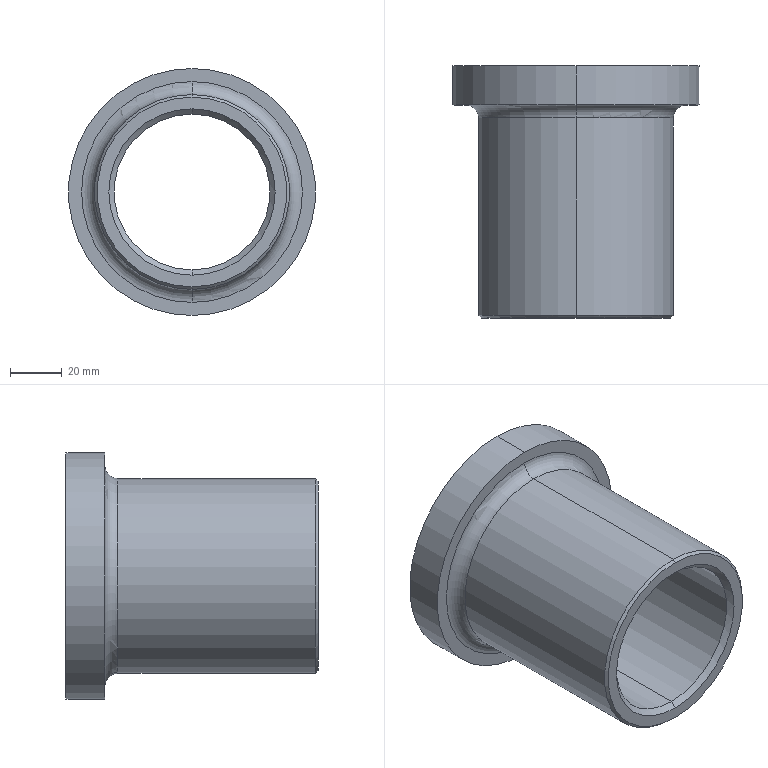Part | SolidWorks | features Chamfer 3, Extrusion 1, Fillet 1, ICE 1 | 1 solid | 17 faces | box 95 x 97 x 95 mm | volume 192640 mm3 | cone 6 | cylinder 6 | plane 3 | torus 2 | commonest cylinder face diameters 60 x2 75 x2 95 x2
STEP:
#1=CARTESIAN_POINT('',(0.,-82.,-36.5));
#2=VERTEX_POINT('',#1);
#3=CARTESIAN_POINT('',(0.,-82.,36.5));
#4=VERTEX_POINT('',#3);
#5=CARTESIAN_POINT('',(0.,-82.,0.));
#6=DIRECTION('',(0.,-1.,0.));
#7=DIRECTION('',(0.,0.,-1.));
#8=AXIS2_PLACEMENT_3D('',#5,#6,#7);
#9=CIRCLE('',#8,36.5);
#10=EDGE_CURVE('',#2,#4,#9,.T.);
#11=ORIENTED_EDGE('',*,*,#10,.F.);
#12=CARTESIAN_POINT('',(0.,-81.,-37.5));
#13=VERTEX_POINT('',#12);
#14=CARTESIAN_POINT('',(0.,-82.,-36.5));
#15=DIRECTION('',(0.,0.7071,-0.7071));
#16=VECTOR('',#15,1000.);
#17=LINE('',#14,#16);
#18=EDGE_CURVE('',#2,#13,#17,.T.);
#19=ORIENTED_EDGE('',*,*,#18,.T.);
#20=CARTESIAN_POINT('',(0.,-81.,37.5));
#21=VERTEX_POINT('',#20);
#22=CARTESIAN_POINT('',(0.,-81.,0.));
#23=DIRECTION('',(0.,1.,0.));
#24=DIRECTION('',(0.,0.,-1.));
#25=AXIS2_PLACEMENT_3D('',#22,#23,#24);
#26=CIRCLE('',#25,37.5);
#27=EDGE_CURVE('',#21,#13,#26,.T.);
#28=ORIENTED_EDGE('',*,*,#27,.F.);
#29=CARTESIAN_POINT('',(0.,-82.,36.5));
#30=DIRECTION('',(0.,0.7071,0.7071));
#31=VECTOR('',#30,1000.);
#32=LINE('',#29,#31);
#33=EDGE_CURVE('',#4,#21,#32,.T.);
#34=ORIENTED_EDGE('',*,*,#33,.F.);
#35=EDGE_LOOP('',(#11,#19,#28,#34));
#36=FACE_OUTER_BOUND('',#35,.T.);
#37=CARTESIAN_POINT('',(0.,-82.,0.));
#38=DIRECTION('',(0.,1.,0.));
#39=DIRECTION('',(0.,0.,1.));
#40=AXIS2_PLACEMENT_3D('',#37,#38,#39);
#41=CONICAL_SURFACE('',#40,36.5,0.7854);
#42=ADVANCED_FACE('',(#36),#41,.T.);
#43=CARTESIAN_POINT('',(0.,10.,-30.));
#44=VERTEX_POINT('',#43);
#45=CARTESIAN_POINT('',(0.,10.,30.));
#46=VERTEX_POINT('',#45);
#47=CARTESIAN_POINT('',(0.,10.,0.));
#48=DIRECTION('',(0.,1.,0.));
#49=DIRECTION('',(0.,0.,1.));
#50=AXIS2_PLACEMENT_3D('',#47,#48,#49);
#51=CIRCLE('',#50,30.);
#52=EDGE_CURVE('',#44,#46,#51,.T.);
#53=ORIENTED_EDGE('',*,*,#52,.F.);
#54=CARTESIAN_POINT('',(0.,15.,-35.));
#55=VERTEX_POINT('',#54);
#56=CARTESIAN_POINT('',(0.,10.,-30.));
#57=DIRECTION('',(0.,0.7071,-0.7071));
#58=VECTOR('',#57,1000.);
#59=LINE('',#56,#58);
#60=EDGE_CURVE('',#44,#55,#59,.T.);
#61=ORIENTED_EDGE('',*,*,#60,.T.);
#62=CARTESIAN_POINT('',(0.,15.,35.));
#63=VERTEX_POINT('',#62);
#64=CARTESIAN_POINT('',(0.,15.,0.));
#65=DIRECTION('',(0.,-1.,0.));
#66=DIRECTION('',(0.,0.,1.));
#67=AXIS2_PLACEMENT_3D('',#64,#65,#66);
#68=CIRCLE('',#67,35.);
#69=EDGE_CURVE('',#63,#55,#68,.T.);
#70=ORIENTED_EDGE('',*,*,#69,.F.);
#71=CARTESIAN_POINT('',(0.,10.,30.));
#72=DIRECTION('',(0.,0.7071,0.7071));
#73=VECTOR('',#72,1000.);
#74=LINE('',#71,#73);
#75=EDGE_CURVE('',#46,#63,#74,.T.);
#76=ORIENTED_EDGE('',*,*,#75,.F.);
#77=EDGE_LOOP('',(#53,#61,#70,#76));
#78=FACE_OUTER_BOUND('',#77,.T.);
#79=CARTESIAN_POINT('',(0.,10.,0.));
#80=DIRECTION('',(0.,1.,0.));
#81=DIRECTION('',(0.,0.,1.));
#82=AXIS2_PLACEMENT_3D('',#79,#80,#81);
#83=CONICAL_SURFACE('',#82,30.,0.7854);
#84=ADVANCED_FACE('',(#78),#83,.F.);
#85=CARTESIAN_POINT('',(0.,-80.,30.));
#86=VERTEX_POINT('',#85);
#87=CARTESIAN_POINT('',(0.,-80.,-30.));
#88=VERTEX_POINT('',#87);
#89=CARTESIAN_POINT('',(0.,-80.,0.));
#90=DIRECTION('',(0.,-1.,0.));
#91=DIRECTION('',(0.,0.,-1.));
#92=AXIS2_PLACEMENT_3D('',#89,#90,#91);
#93=CIRCLE('',#92,30.);
#94=EDGE_CURVE('',#86,#88,#93,.T.);
#95=ORIENTED_EDGE('',*,*,#94,.F.);
#96=CARTESIAN_POINT('',(0.,-82.,32.));
#97=VERTEX_POINT('',#96);
#98=CARTESIAN_POINT('',(0.,-80.,30.));
#99=DIRECTION('',(0.,-0.7071,0.7071));
#100=VECTOR('',#99,1000.);
#101=LINE('',#98,#100);
#102=EDGE_CURVE('',#86,#97,#101,.T.);
#103=ORIENTED_EDGE('',*,*,#102,.T.);
#104=CARTESIAN_POINT('',(0.,-82.,-32.));
#105=VERTEX_POINT('',#104);
#106=CARTESIAN_POINT('',(0.,-82.,0.));
#107=DIRECTION('',(0.,1.,0.));
#108=DIRECTION('',(0.,0.,-1.));
#109=AXIS2_PLACEMENT_3D('',#106,#107,#108);
#110=CIRCLE('',#109,32.);
#111=EDGE_CURVE('',#105,#97,#110,.T.);
#112=ORIENTED_EDGE('',*,*,#111,.F.);
#113=CARTESIAN_POINT('',(0.,-80.,-30.));
#114=DIRECTION('',(0.,-0.7071,-0.7071));
#115=VECTOR('',#114,1000.);
#116=LINE('',#113,#115);
#117=EDGE_CURVE('',#88,#105,#116,.T.);
#118=ORIENTED_EDGE('',*,*,#117,.F.);
#119=EDGE_LOOP('',(#95,#103,#112,#118));
#120=FACE_OUTER_BOUND('',#119,.T.);
#121=CARTESIAN_POINT('',(0.,-80.,0.));
#122=DIRECTION('',(0.,-1.,0.));
#123=DIRECTION('',(0.,0.,-1.));
#124=AXIS2_PLACEMENT_3D('',#121,#122,#123);
#125=CONICAL_SURFACE('',#124,30.,0.7854);
#126=ADVANCED_FACE('',(#120),#125,.F.);
#127=CARTESIAN_POINT('',(0.,0.,-42.5));
#128=VERTEX_POINT('',#127);
#129=CARTESIAN_POINT('',(0.,0.,42.5));
#130=VERTEX_POINT('',#129);
#131=CARTESIAN_POINT('',(0.,0.,0.));
#132=DIRECTION('',(0.,1.,0.));
#133=DIRECTION('',(0.,0.,1.));
#134=AXIS2_PLACEMENT_3D('',#131,#132,#133);
#135=CIRCLE('',#134,42.5);
#136=EDGE_CURVE('',#128,#130,#135,.T.);
#137=ORIENTED_EDGE('',*,*,#136,.F.);
#138=CARTESIAN_POINT('',(0.,-5.,-37.5));
#139=VERTEX_POINT('',#138);
#140=CARTESIAN_POINT('',(0.,-5.,-42.5));
#141=DIRECTION('',(1.,0.,0.));
#142=DIRECTION('',(0.,0.,-1.));
#143=AXIS2_PLACEMENT_3D('',#140,#141,#142);
#144=CIRCLE('',#143,5.);
#145=EDGE_CURVE('',#128,#139,#144,.T.);
#146=ORIENTED_EDGE('',*,*,#145,.T.);
#147=CARTESIAN_POINT('',(0.,-5.,37.5));
#148=VERTEX_POINT('',#147);
#149=CARTESIAN_POINT('',(0.,-5.,0.));
#150=DIRECTION('',(0.,-1.,0.));
#151=DIRECTION('',(0.,0.,1.));
#152=AXIS2_PLACEMENT_3D('',#149,#150,#151);
#153=CIRCLE('',#152,37.5);
#154=EDGE_CURVE('',#148,#139,#153,.T.);
#155=ORIENTED_EDGE('',*,*,#154,.F.);
#156=CARTESIAN_POINT('',(0.,-5.,42.5));
#157=DIRECTION('',(-1.,0.,0.));
#158=DIRECTION('',(0.,0.,1.));
#159=AXIS2_PLACEMENT_3D('',#156,#157,#158);
#160=CIRCLE('',#159,5.);
#161=EDGE_CURVE('',#130,#148,#160,.T.);
#162=ORIENTED_EDGE('',*,*,#161,.F.);
#163=EDGE_LOOP('',(#137,#146,#155,#162));
#164=FACE_OUTER_BOUND('',#163,.T.);
#165=CARTESIAN_POINT('',(0.,-5.,0.));
#166=DIRECTION('',(0.,1.,0.));
#167=DIRECTION('',(0.,0.,1.));
#168=AXIS2_PLACEMENT_3D('',#165,#166,#167);
#169=TOROIDAL_SURFACE('',#168,42.5,5.);
#170=ADVANCED_FACE('',(#164),#169,.F.);
#171=ORIENTED_EDGE('',*,*,#27,.T.);
#172=CARTESIAN_POINT('',(0.,-82.,-37.5));
#173=DIRECTION('',(0.,1.,0.));
#174=VECTOR('',#173,1000.);
#175=LINE('',#172,#174);
#176=EDGE_CURVE('',#13,#139,#175,.T.);
#177=ORIENTED_EDGE('',*,*,#176,.T.);
#178=CARTESIAN_POINT('',(0.,-5.,0.));
#179=DIRECTION('',(0.,-1.,0.));
#180=DIRECTION('',(0.,0.,1.));
#181=AXIS2_PLACEMENT_3D('',#178,#179,#180);
#182=CIRCLE('',#181,37.5);
#183=EDGE_CURVE('',#139,#148,#182,.T.);
#184=ORIENTED_EDGE('',*,*,#183,.T.);
#185=CARTESIAN_POINT('',(0.,-82.,37.5));
#186=DIRECTION('',(0.,1.,0.));
#187=VECTOR('',#186,1000.);
#188=LINE('',#185,#187);
#189=EDGE_CURVE('',#21,#148,#188,.T.);
#190=ORIENTED_EDGE('',*,*,#189,.F.);
#191=EDGE_LOOP('',(#171,#177,#184,#190));
#192=FACE_OUTER_BOUND('',#191,.T.);
#193=CARTESIAN_POINT('',(0.,-82.,0.));
#194=DIRECTION('',(0.,1.,0.));
#195=DIRECTION('',(0.,0.,1.));
#196=AXIS2_PLACEMENT_3D('',#193,#194,#195);
#197=CYLINDRICAL_SURFACE('',#196,37.5);
#198=ADVANCED_FACE('',(#192),#197,.T.);
#199=ORIENTED_EDGE('',*,*,#52,.T.);
#200=CARTESIAN_POINT('',(0.,15.,30.));
#201=DIRECTION('',(0.,-1.,0.));
#202=VECTOR('',#201,1000.);
#203=LINE('',#200,#202);
#204=EDGE_CURVE('',#46,#86,#203,.T.);
#205=ORIENTED_EDGE('',*,*,#204,.T.);
#206=ORIENTED_EDGE('',*,*,#94,.T.);
#207=CARTESIAN_POINT('',(0.,15.,-30.));
#208=DIRECTION('',(0.,-1.,0.));
#209=VECTOR('',#208,1000.);
#210=LINE('',#207,#209);
#211=EDGE_CURVE('',#44,#88,#210,.T.);
#212=ORIENTED_EDGE('',*,*,#211,.F.);
#213=EDGE_LOOP('',(#199,#205,#206,#212));
#214=FACE_OUTER_BOUND('',#213,.T.);
#215=CARTESIAN_POINT('',(0.,15.,0.));
#216=DIRECTION('',(0.,-1.,0.));
#217=DIRECTION('',(0.,0.,-1.));
#218=AXIS2_PLACEMENT_3D('',#215,#216,#217);
#219=CYLINDRICAL_SURFACE('',#218,30.);
#220=ADVANCED_FACE('',(#214),#219,.F.);
#221=CARTESIAN_POINT('',(0.,15.,47.5));
#222=VERTEX_POINT('',#221);
#223=CARTESIAN_POINT('',(0.,15.,-47.5));
#224=VERTEX_POINT('',#223);
#225=CARTESIAN_POINT('',(0.,15.,0.));
#226=DIRECTION('',(0.,1.,0.));
#227=DIRECTION('',(0.,0.,1.));
#228=AXIS2_PLACEMENT_3D('',#225,#226,#227);
#229=CIRCLE('',#228,47.5);
#230=EDGE_CURVE('',#222,#224,#229,.T.);
#231=ORIENTED_EDGE('',*,*,#230,.F.);
#232=CARTESIAN_POINT('',(0.,0.,47.5));
#233=VERTEX_POINT('',#232);
#234=CARTESIAN_POINT('',(0.,15.,47.5));
#235=DIRECTION('',(0.,-1.,0.));
#236=VECTOR('',#235,1000.);
#237=LINE('',#234,#236);
#238=EDGE_CURVE('',#222,#233,#237,.T.);
#239=ORIENTED_EDGE('',*,*,#238,.T.);
#240=CARTESIAN_POINT('',(0.,0.,-47.5));
#241=VERTEX_POINT('',#240);
#242=CARTESIAN_POINT('',(0.,0.,0.));
#243=DIRECTION('',(0.,1.,0.));
#244=DIRECTION('',(0.,0.,1.));
#245=AXIS2_PLACEMENT_3D('',#242,#243,#244);
#246=CIRCLE('',#245,47.5);
#247=EDGE_CURVE('',#233,#241,#246,.T.);
#248=ORIENTED_EDGE('',*,*,#247,.T.);
#249=CARTESIAN_POINT('',(0.,15.,-47.5));
#250=DIRECTION('',(0.,-1.,0.));
#251=VECTOR('',#250,1000.);
#252=LINE('',#249,#251);
#253=EDGE_CURVE('',#224,#241,#252,.T.);
#254=ORIENTED_EDGE('',*,*,#253,.F.);
#255=EDGE_LOOP('',(#231,#239,#248,#254));
#256=FACE_OUTER_BOUND('',#255,.T.);
#257=CARTESIAN_POINT('',(0.,15.,0.));
#258=DIRECTION('',(0.,-1.,0.));
#259=DIRECTION('',(0.,0.,-1.));
#260=AXIS2_PLACEMENT_3D('',#257,#258,#259);
#261=CYLINDRICAL_SURFACE('',#260,47.5);
#262=ADVANCED_FACE('',(#256),#261,.T.);
#263=CARTESIAN_POINT('',(0.,0.,0.));
#264=DIRECTION('',(0.,1.,0.));
#265=DIRECTION('',(0.,0.,1.));
#266=AXIS2_PLACEMENT_3D('',#263,#264,#265);
#267=CIRCLE('',#266,42.5);
#268=EDGE_CURVE('',#130,#128,#267,.T.);
#269=ORIENTED_EDGE('',*,*,#268,.T.);
#270=ORIENTED_EDGE('',*,*,#136,.T.);
#271=EDGE_LOOP('',(#269,#270));
#272=FACE_BOUND('',#271,.T.);
#273=CARTESIAN_POINT('',(0.,0.,0.));
#274=DIRECTION('',(0.,1.,0.));
#275=DIRECTION('',(0.,0.,1.));
#276=AXIS2_PLACEMENT_3D('',#273,#274,#275);
#277=CIRCLE('',#276,47.5);
#278=EDGE_CURVE('',#241,#233,#277,.T.);
#279=ORIENTED_EDGE('',*,*,#278,.F.);
#280=ORIENTED_EDGE('',*,*,#247,.F.);
#281=EDGE_LOOP('',(#279,#280));
#282=FACE_OUTER_BOUND('',#281,.T.);
#283=CARTESIAN_POINT('',(0.,0.,0.));
#284=DIRECTION('',(0.,1.,0.));
#285=DIRECTION('',(0.,0.,1.));
#286=AXIS2_PLACEMENT_3D('',#283,#284,#285);
#287=PLANE('',#286);
#288=ADVANCED_FACE('',(#272,#282),#287,.F.);
#289=ORIENTED_EDGE('',*,*,#69,.T.);
#290=CARTESIAN_POINT('',(0.,15.,0.));
#291=DIRECTION('',(0.,-1.,0.));
#292=DIRECTION('',(0.,0.,1.));
#293=AXIS2_PLACEMENT_3D('',#290,#291,#292);
#294=CIRCLE('',#293,35.);
#295=EDGE_CURVE('',#55,#63,#294,.T.);
#296=ORIENTED_EDGE('',*,*,#295,.T.);
#297=EDGE_LOOP('',(#289,#296));
#298=FACE_BOUND('',#297,.T.);
#299=CARTESIAN_POINT('',(0.,15.,0.));
#300=DIRECTION('',(0.,1.,0.));
#301=DIRECTION('',(0.,0.,1.));
#302=AXIS2_PLACEMENT_3D('',#299,#300,#301);
#303=CIRCLE('',#302,47.5);
#304=EDGE_CURVE('',#224,#222,#303,.T.);
#305=ORIENTED_EDGE('',*,*,#304,.T.);
#306=ORIENTED_EDGE('',*,*,#230,.T.);
#307=EDGE_LOOP('',(#305,#306));
#308=FACE_OUTER_BOUND('',#307,.T.);
#309=CARTESIAN_POINT('',(0.,15.,0.));
#310=DIRECTION('',(0.,1.,0.));
#311=DIRECTION('',(0.,0.,1.));
#312=AXIS2_PLACEMENT_3D('',#309,#310,#311);
#313=PLANE('',#312);
#314=ADVANCED_FACE('',(#298,#308),#313,.T.);
#315=ORIENTED_EDGE('',*,*,#238,.F.);
#316=ORIENTED_EDGE('',*,*,#304,.F.);
#317=ORIENTED_EDGE('',*,*,#253,.T.);
#318=ORIENTED_EDGE('',*,*,#278,.T.);
#319=EDGE_LOOP('',(#315,#316,#317,#318));
#320=FACE_OUTER_BOUND('',#319,.T.);
#321=CARTESIAN_POINT('',(0.,15.,0.));
#322=DIRECTION('',(0.,-1.,0.));
#323=DIRECTION('',(0.,0.,-1.));
#324=AXIS2_PLACEMENT_3D('',#321,#322,#323);
#325=CYLINDRICAL_SURFACE('',#324,47.5);
#326=ADVANCED_FACE('',(#320),#325,.T.);
#327=ORIENTED_EDGE('',*,*,#204,.F.);
#328=CARTESIAN_POINT('',(0.,10.,0.));
#329=DIRECTION('',(0.,1.,0.));
#330=DIRECTION('',(0.,0.,1.));
#331=AXIS2_PLACEMENT_3D('',#328,#329,#330);
#332=CIRCLE('',#331,30.);
#333=EDGE_CURVE('',#46,#44,#332,.T.);
#334=ORIENTED_EDGE('',*,*,#333,.T.);
#335=ORIENTED_EDGE('',*,*,#211,.T.);
#336=CARTESIAN_POINT('',(0.,-80.,0.));
#337=DIRECTION('',(0.,-1.,0.));
#338=DIRECTION('',(0.,0.,-1.));
#339=AXIS2_PLACEMENT_3D('',#336,#337,#338);
#340=CIRCLE('',#339,30.);
#341=EDGE_CURVE('',#88,#86,#340,.T.);
#342=ORIENTED_EDGE('',*,*,#341,.T.);
#343=EDGE_LOOP('',(#327,#334,#335,#342));
#344=FACE_OUTER_BOUND('',#343,.T.);
#345=CARTESIAN_POINT('',(0.,15.,0.));
#346=DIRECTION('',(0.,-1.,0.));
#347=DIRECTION('',(0.,0.,-1.));
#348=AXIS2_PLACEMENT_3D('',#345,#346,#347);
#349=CYLINDRICAL_SURFACE('',#348,30.);
#350=ADVANCED_FACE('',(#344),#349,.F.);
#351=CARTESIAN_POINT('',(0.,-82.,0.));
#352=DIRECTION('',(0.,-1.,0.));
#353=DIRECTION('',(0.,0.,-1.));
#354=AXIS2_PLACEMENT_3D('',#351,#352,#353);
#355=CIRCLE('',#354,36.5);
#356=EDGE_CURVE('',#4,#2,#355,.T.);
#357=ORIENTED_EDGE('',*,*,#356,.T.);
#358=ORIENTED_EDGE('',*,*,#10,.T.);
#359=EDGE_LOOP('',(#357,#358));
#360=FACE_OUTER_BOUND('',#359,.T.);
#361=ORIENTED_EDGE('',*,*,#111,.T.);
#362=CARTESIAN_POINT('',(0.,-82.,0.));
#363=DIRECTION('',(0.,1.,0.));
#364=DIRECTION('',(0.,0.,-1.));
#365=AXIS2_PLACEMENT_3D('',#362,#363,#364);
#366=CIRCLE('',#365,32.);
#367=EDGE_CURVE('',#97,#105,#366,.T.);
#368=ORIENTED_EDGE('',*,*,#367,.T.);
#369=EDGE_LOOP('',(#361,#368));
#370=FACE_BOUND('',#369,.T.);
#371=CARTESIAN_POINT('',(0.,-82.,0.));
#372=DIRECTION('',(0.,-1.,0.));
#373=DIRECTION('',(0.,0.,-1.));
#374=AXIS2_PLACEMENT_3D('',#371,#372,#373);
#375=PLANE('',#374);
#376=ADVANCED_FACE('',(#360,#370),#375,.T.);
#377=ORIENTED_EDGE('',*,*,#176,.F.);
#378=CARTESIAN_POINT('',(0.,-81.,0.));
#379=DIRECTION('',(0.,1.,0.));
#380=DIRECTION('',(0.,0.,-1.));
#381=AXIS2_PLACEMENT_3D('',#378,#379,#380);
#382=CIRCLE('',#381,37.5);
#383=EDGE_CURVE('',#13,#21,#382,.T.);
#384=ORIENTED_EDGE('',*,*,#383,.T.);
#385=ORIENTED_EDGE('',*,*,#189,.T.);
#386=ORIENTED_EDGE('',*,*,#154,.T.);
#387=EDGE_LOOP('',(#377,#384,#385,#386));
#388=FACE_OUTER_BOUND('',#387,.T.);
#389=CARTESIAN_POINT('',(0.,-82.,0.));
#390=DIRECTION('',(0.,1.,0.));
#391=DIRECTION('',(0.,0.,1.));
#392=AXIS2_PLACEMENT_3D('',#389,#390,#391);
#393=CYLINDRICAL_SURFACE('',#392,37.5);
#394=ADVANCED_FACE('',(#388),#393,.T.);
#395=ORIENTED_EDGE('',*,*,#145,.F.);
#396=ORIENTED_EDGE('',*,*,#268,.F.);
#397=ORIENTED_EDGE('',*,*,#161,.T.);
#398=ORIENTED_EDGE('',*,*,#183,.F.);
#399=EDGE_LOOP('',(#395,#396,#397,#398));
#400=FACE_OUTER_BOUND('',#399,.T.);
#401=CARTESIAN_POINT('',(0.,-5.,0.));
#402=DIRECTION('',(0.,1.,0.));
#403=DIRECTION('',(0.,0.,1.));
#404=AXIS2_PLACEMENT_3D('',#401,#402,#403);
#405=TOROIDAL_SURFACE('',#404,42.5,5.);
#406=ADVANCED_FACE('',(#400),#405,.F.);
#407=ORIENTED_EDGE('',*,*,#102,.F.);
#408=ORIENTED_EDGE('',*,*,#341,.F.);
#409=ORIENTED_EDGE('',*,*,#117,.T.);
#410=ORIENTED_EDGE('',*,*,#367,.F.);
#411=EDGE_LOOP('',(#407,#408,#409,#410));
#412=FACE_OUTER_BOUND('',#411,.T.);
#413=CARTESIAN_POINT('',(0.,-80.,0.));
#414=DIRECTION('',(0.,-1.,0.));
#415=DIRECTION('',(0.,0.,-1.));
#416=AXIS2_PLACEMENT_3D('',#413,#414,#415);
#417=CONICAL_SURFACE('',#416,30.,0.7854);
#418=ADVANCED_FACE('',(#412),#417,.F.);
#419=ORIENTED_EDGE('',*,*,#60,.F.);
#420=ORIENTED_EDGE('',*,*,#333,.F.);
#421=ORIENTED_EDGE('',*,*,#75,.T.);
#422=ORIENTED_EDGE('',*,*,#295,.F.);
#423=EDGE_LOOP('',(#419,#420,#421,#422));
#424=FACE_OUTER_BOUND('',#423,.T.);
#425=CARTESIAN_POINT('',(0.,10.,0.));
#426=DIRECTION('',(0.,1.,0.));
#427=DIRECTION('',(0.,0.,1.));
#428=AXIS2_PLACEMENT_3D('',#425,#426,#427);
#429=CONICAL_SURFACE('',#428,30.,0.7854);
#430=ADVANCED_FACE('',(#424),#429,.F.);
#431=ORIENTED_EDGE('',*,*,#18,.F.);
#432=ORIENTED_EDGE('',*,*,#356,.F.);
#433=ORIENTED_EDGE('',*,*,#33,.T.);
#434=ORIENTED_EDGE('',*,*,#383,.F.);
#435=EDGE_LOOP('',(#431,#432,#433,#434));
#436=FACE_OUTER_BOUND('',#435,.T.);
#437=CARTESIAN_POINT('',(0.,-82.,0.));
#438=DIRECTION('',(0.,1.,0.));
#439=DIRECTION('',(0.,0.,1.));
#440=AXIS2_PLACEMENT_3D('',#437,#438,#439);
#441=CONICAL_SURFACE('',#440,36.5,0.7854);
#442=ADVANCED_FACE('',(#436),#441,.T.);
#443=CLOSED_SHELL('',(#42,#84,#126,#170,#198,#220,#262,#288,#314,#326,#350,#376,#394,#406,#418,#430,#442));
#444=MANIFOLD_SOLID_BREP('',#443);
#445=CARTESIAN_POINT('',(0.,0.,0.));
#446=DIRECTION('',(0.,0.,1.));
#447=DIRECTION('',(1.,0.,0.));
#448=AXIS2_PLACEMENT_3D('',#445,#446,#447);
#449=(LENGTH_UNIT()NAMED_UNIT(*)SI_UNIT(.MILLI.,.METRE.));
#450=UNCERTAINTY_MEASURE_WITH_UNIT(LENGTH_MEASURE(0.00001),#449,'','');
#451=(NAMED_UNIT(*)PLANE_ANGLE_UNIT()SI_UNIT($,.RADIAN.));
#452=(NAMED_UNIT(*)SI_UNIT($,.STERADIAN.)SOLID_ANGLE_UNIT());
#453=(GEOMETRIC_REPRESENTATION_CONTEXT(3)GLOBAL_UNCERTAINTY_ASSIGNED_CONTEXT((#450))GLOBAL_UNIT_ASSIGNED_CONTEXT((#449,#451,#452))REPRESENTATION_CONTEXT('',''));
#454=ADVANCED_BREP_SHAPE_REPRESENTATION('',(#444,#448),#453);